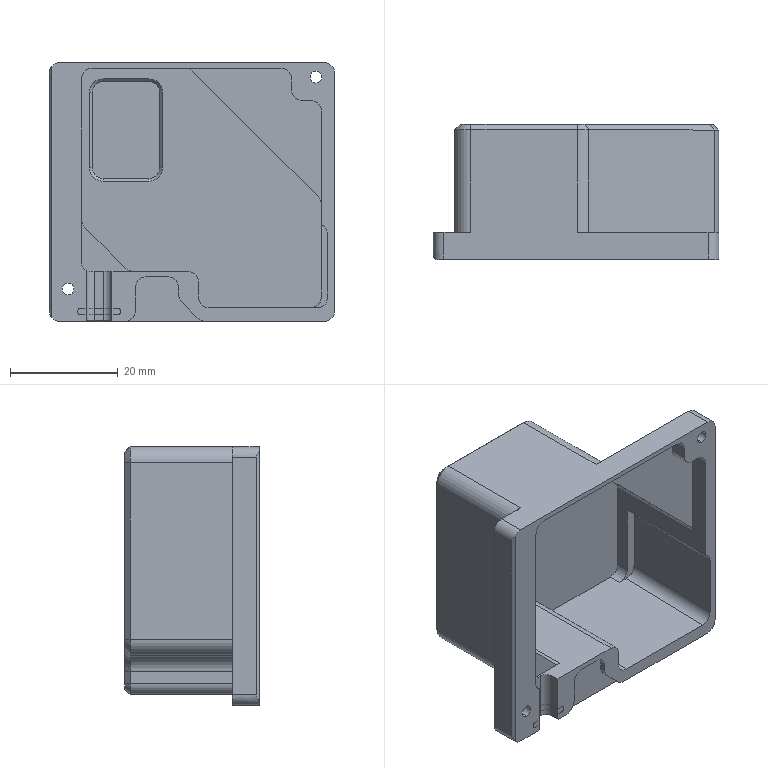CAM job | NX | 3+2 milling, drilling | part box 53 x 25 x 48 mm | stock box 58 x 35 x 53 mm
Tools:
number,name,description,diameter,corner_radius,flute_length,length,flutes
12,D1-10-D4-50-3T,D1*10*4*50-3T,1.0,0.0,10.0,11.0,3
10,D2-6-D4-50-3T-ROUGH,D2-6-D4-50-3T-粗,2.0,0.0,6.0,7.0,2
4,D3-9-D4-50-3T-FINISH,D3-9-D4-50-3T-精,3.0,0.0,9.0,10.0,2
9,D4-12-D4-50-3T-ROUGH,D4-12-D4-50-3T-粗,4.0,0.0,12.0,50.0,2
13,D4-12-D4-50-3T-FINISH,D4-12-D4-50-3T,4.0,0.0,12.0,50.0,3
3,D6-18-D6-50-3T-ROUGH,D6-18-D6-50-3T-粗,6.0,0.0,18.0,50.0,2
2,D10-30-D10-75-3T-ROUGH,D10-30-D10-75-3T-粗,10.0,0.0,30.0,75.0,2
5,D10-30-D10-75-3T-FINISH,D10-30-D10-75-3T,10.0,0.0,30.0,75.0,3
1,D63面刀,D63面刀,63.0,0.0,30.0,30.0,4
14,倒角D3-90度,倒角D3-90度,3.0,0.0,5.0,50.0,2
6,倒角D6-90度,倒角D6-90度,6.0,0.0,5.0,50.0,2
8,球刀R0.5-2-D4-50,球刀R0.5-2-D4-50,1.0,0.5,2.0,2.5,2
11,球刀R0.75-3-D4-50,球刀R0.75-3-D4-50,1.5,0.75,3.0,10.0,2
7,D2.2钻头,Drilling Tool,2.2,0.0,35.0,50.0,2
Operations:
program,operation,operation_type,tool,method,geometry_group,spindle_rpm,surface_speed,feed_per_tooth,feed_cut,feed_plunge,cut_length_mm,path_length_mm,cut_time_min,machine_time_min
A1,PLANAR_MILL,PlanarMilling,D63面刀,METHOD,A-G54,3500.0,692.0,0.0571,1000.0,100.0,882.0,1948.8,0.882,0.9887
A1,动态粗,CavityMilling,D10-30-D10-75-3T-ROUGH,METHOD,WORKPIECE_54,5500.0,172.0,0.2727,3000.0,100.0,2155.931,2536.016,0.6891,0.7271
A1,动态粗_COPY,CavityMilling,D6-18-D6-50-3T-ROUGH,METHOD,WORKPIECE_54,5500.0,103.0,0.1818,2000.0,100.0,48.224,232.95,0.0241,0.0426
A1,FLOOR_FACING,VolumeBased25DMillingOperation,D6-18-D6-50-3T-ROUGH,METHOD,WORKPIECE_54,4500.0,84.0,0.1111,1000.0,100.0,387.029,441.429,0.387,0.3925
A1,FLOOR_FACING_COPY,VolumeBased25DMillingOperation,D6-18-D6-50-3T-ROUGH,METHOD,WORKPIECE_54,4500.0,84.0,0.0889,800.0,100.0,387.029,441.629,0.4838,0.4892
A1,PLANAR_MILL_1_COPY_COPY,PlanarMilling,D6-18-D6-50-3T-ROUGH,METHOD,WORKPIECE_54,4500.0,84.0,0.0667,600.0,100.0,83.665,264.157,0.1394,0.1575
A1,FLOOR_FACING_COPY_COPY,VolumeBased25DMillingOperation,D3-9-D4-50-3T-FINISH,METHOD,WORKPIECE_54,4500.0,42.0,0.0889,800.0,100.0,153.436,210.036,0.1918,0.1975
A1,PLANAR_MILL_4,PlanarMilling,D10-30-D10-75-3T-FINISH,METHOD,A-G54,4500.0,141.0,0.0593,800.0,100.0,158.007,214.007,0.1975,0.2031
A1,PLANAR_MILL_1,PlanarMilling,D10-30-D10-75-3T-FINISH,METHOD,WORKPIECE_54,5500.0,172.0,0.0364,600.0,100.0,480.531,588.531,0.8009,0.8117
A1,PLANAR_MILL_1_COPY,PlanarMilling,D10-30-D10-75-3T-FINISH,METHOD,WORKPIECE_54,4500.0,141.0,0.0593,800.0,100.0,366.253,884.576,0.4578,0.5096
A1,PLANAR_MILL_1_COPY_COPY_1,PlanarMilling,D10-30-D10-75-3T-FINISH,METHOD,WORKPIECE_54,4500.0,141.0,0.0593,800.0,100.0,50.908,312.799,0.0636,0.0898
A1,PLANAR_MILL_2,PlanarMilling,倒角D6-90度,METHOD,WORKPIECE_54,3500.0,65.0,0.1143,800.0,100.0,182.942,241.942,0.2287,0.2346
A1,PLANAR_MILL_2_COPY,PlanarMilling,倒角D6-90度,METHOD,WORKPIECE_54,3500.0,65.0,0.1143,800.0,100.0,172.416,400.7,0.2155,0.2383
A1,DRILLING,Operation,倒角D6-90度,METHOD,WORKPIECE_54,3000.0,56.0,0.0333,200.0,0.0,10.4,184.376,0.052,0.0694
A1,DRILLING_COPY,Operation,D2.2钻头,METHOD,WORKPIECE_54,3000.0,20.0,0.025,150.0,0.0,21.0,205.576,0.14,0.1585
A1,HOLE_MILLING,CylinderMilling,D3-9-D4-50-3T-FINISH,METHOD,WORKPIECE_54,4500.0,42.0,0.0333,300.0,100.0,123.264,386.766,0.4109,0.4372
A1,PLANAR_MILL_2_COPY_1,PlanarMilling,球刀R0.5-2-D4-50,METHOD,WORKPIECE_54,3500.0,10.0,0.1143,800.0,100.0,159.924,216.324,0.1999,0.2055
B1,动态粗_COPY_1,CavityMilling,D10-30-D10-75-3T-ROUGH,METHOD,WORKPIECE_55,6500.0,204.0,0.1538,2000.0,100.0,5076.554,5135.254,2.538,2.544
B1,动态粗_COPY_1_COPY,CavityMilling,D10-30-D10-75-3T-ROUGH,METHOD,WORKPIECE_55,6500.0,204.0,0.1538,2000.0,100.0,4756.895,5114.723,2.361,2.396
B1,PLANAR_MILL_3,PlanarMilling,D4-12-D4-50-3T-ROUGH,METHOD,B-G55,3000.0,37.0,0.1,600.0,100.0,2155.972,3366.3,3.593,3.714
B1,PLANAR_MILL_3_COPY_COPY,PlanarMilling,D4-12-D4-50-3T-ROUGH,METHOD,B-G55,3000.0,37.0,0.1,600.0,100.0,361.385,602.012,0.6023,0.6264
B1,PLANAR_MILL_3_COPY_COPY_COPY,PlanarMilling,D4-12-D4-50-3T-ROUGH,METHOD,B-G55,3000.0,37.0,0.1,600.0,100.0,86.344,145.356,0.1439,0.1498
B1,PLANAR_MILL_3_COPY,PlanarMilling,D4-12-D4-50-3T-ROUGH,METHOD,B-G55,4500.0,56.0,0.0667,600.0,100.0,379.272,493.874,0.6321,0.6436
B1,CAVITY_MILL_1,CavityMilling,D2-6-D4-50-3T-ROUGH,METHOD,WORKPIECE,6500.0,40.0,0.0923,1200.0,100.0,1076.502,1197.623,0.8971,0.9092
B1,PLANAR_MILL_9,PlanarMilling,D2-6-D4-50-3T-ROUGH,METHOD,B-G55,4500.0,28.0,0.0333,300.0,100.0,83.489,164.661,0.2783,0.2864
B1,AREA_MILL,SurfaceContour,球刀R0.75-3-D4-50,METHOD,WORKPIECE,6500.0,30.0,0.1538,2000.0,100.0,1524.697,1762.314,0.7623,0.7861
B1,PLANAR_MILL_5,PlanarMilling,D10-30-D10-75-3T-FINISH,METHOD,B-G55,4500.0,141.0,0.0593,800.0,100.0,218.245,272.245,0.2728,0.2782
B1,PLANAR_MILL_5_COPY,PlanarMilling,D10-30-D10-75-3T-FINISH,METHOD,B-G55,4500.0,141.0,0.0593,800.0,100.0,34.142,90.142,0.0427,0.0483
B1,PLANAR_MILL_6,PlanarMilling,D1-10-D4-50-3T,METHOD,B-G55,6500.0,20.0,0.0103,200.0,100.0,582.435,644.385,2.912,2.918
B1,FLOOR_FACING_1,VolumeBased25DMillingOperation,D4-12-D4-50-3T-FINISH,METHOD,B-G55,3500.0,43.0,0.0571,600.0,100.0,241.102,540.712,0.4018,0.4318
B1,PLANAR_MILL_7,PlanarMilling,D4-12-D4-50-3T-FINISH,METHOD,B-G55,3500.0,43.0,0.0571,600.0,100.0,595.888,699.888,0.9931,1.004
B1,FLOOR_FACING_1_COPY,VolumeBased25DMillingOperation,D4-12-D4-50-3T-FINISH,METHOD,B-G55,3500.0,43.0,0.0571,600.0,100.0,88.507,194.507,0.1475,0.1581
B1,PLANAR_MILL_7_COPY,PlanarMilling,D4-12-D4-50-3T-FINISH,METHOD,B-G55,3500.0,43.0,0.0571,600.0,100.0,902.769,1162.689,1.505,1.531
B1,PLANAR_MILL_7_COPY_COPY,PlanarMilling,D4-12-D4-50-3T-FINISH,METHOD,B-G55,3500.0,43.0,0.0571,600.0,100.0,106.566,210.566,0.1776,0.188
B1,PLANAR_MILL_7_COPY_COPY_COPY,PlanarMilling,D4-12-D4-50-3T-FINISH,METHOD,B-G55,3500.0,43.0,0.0571,600.0,100.0,161.126,480.936,0.2685,0.3005
B1,PLANAR_MILL_7_COPY_COPY_COPY_COPY,PlanarMilling,D4-12-D4-50-3T-FINISH,METHOD,B-G55,3500.0,43.0,0.0571,600.0,100.0,73.207,208.235,0.122,0.1355
B1,PLANAR_MILL_8,PlanarMilling,倒角D3-90度,METHOD,B-G55,3500.0,32.0,0.1143,800.0,100.0,220.979,278.979,0.2762,0.282
B1,PLANAR_MILL_8_COPY,PlanarMilling,倒角D3-90度,METHOD,B-G55,3500.0,32.0,0.1143,800.0,100.0,186.059,244.059,0.2326,0.2384
B1,PLANAR_MILL_8_COPY_COPY,PlanarMilling,倒角D3-90度,METHOD,B-G55,3500.0,32.0,0.1143,800.0,100.0,50.574,211.429,0.0632,0.0793
B1,PLANAR_MILL_8_COPY_COPY_COPY,PlanarMilling,倒角D3-90度,METHOD,B-G55,3500.0,32.0,0.1143,800.0,100.0,121.133,225.133,0.1514,0.1618
C1,ZLEVEL_PROFILE_STEEP,ZLevelMilling,D4-12-D4-50-3T-ROUGH,METHOD,C-G56,4000.0,50.0,0.1875,1500.0,100.0,6034.99,6116.093,4.023,4.031